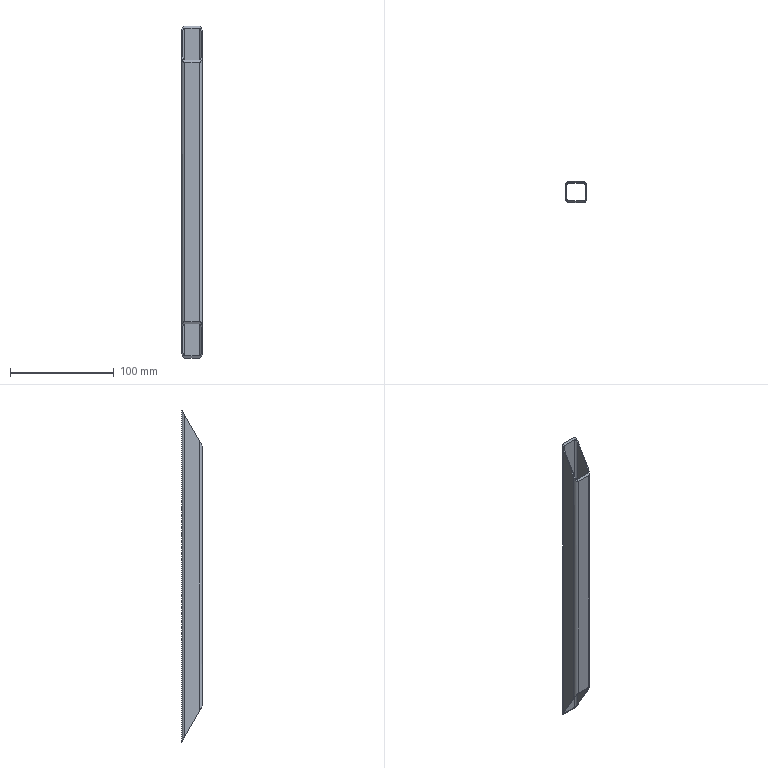Part | SolidWorks | features BaseBody 1 | 1 solid | 18 faces | box 20 x 20 x 320.082 mm | volume 24308 mm3 | plane 10 | cylinder 8 | commonest cylinder face diameters 3.6 x4 6 x4
STEP:
#1=CARTESIAN_POINT('',(7.,10.,0.));
#2=VERTEX_POINT('',#1);
#3=CARTESIAN_POINT('',(-7.,10.,0.));
#4=VERTEX_POINT('',#3);
#5=CARTESIAN_POINT('',(-7.,10.,0.));
#6=DIRECTION('',(-1.,0.,0.));
#7=VECTOR('',#6,1000.);
#8=LINE('',#5,#7);
#9=EDGE_CURVE('',#2,#4,#8,.T.);
#10=ORIENTED_EDGE('',*,*,#9,.T.);
#11=CARTESIAN_POINT('',(-7.,10.,320.082));
#12=VERTEX_POINT('',#11);
#13=CARTESIAN_POINT('',(-7.,10.,0.));
#14=DIRECTION('',(0.,0.,1.));
#15=VECTOR('',#14,1000.);
#16=LINE('',#13,#15);
#17=EDGE_CURVE('',#4,#12,#16,.T.);
#18=ORIENTED_EDGE('',*,*,#17,.T.);
#19=CARTESIAN_POINT('',(7.,10.,320.082));
#20=VERTEX_POINT('',#19);
#21=CARTESIAN_POINT('',(-7.,10.,320.082));
#22=DIRECTION('',(1.,0.,0.));
#23=VECTOR('',#22,1000.);
#24=LINE('',#21,#23);
#25=EDGE_CURVE('',#12,#20,#24,.T.);
#26=ORIENTED_EDGE('',*,*,#25,.T.);
#27=CARTESIAN_POINT('',(7.,10.,0.));
#28=DIRECTION('',(0.,0.,-1.));
#29=VECTOR('',#28,1000.);
#30=LINE('',#27,#29);
#31=EDGE_CURVE('',#20,#2,#30,.T.);
#32=ORIENTED_EDGE('',*,*,#31,.T.);
#33=EDGE_LOOP('',(#10,#18,#26,#32));
#34=FACE_OUTER_BOUND('',#33,.T.);
#35=CARTESIAN_POINT('',(-7.,10.,0.));
#36=DIRECTION('',(0.,1.,0.));
#37=DIRECTION('',(-1.,0.,0.));
#38=AXIS2_PLACEMENT_3D('',#35,#36,#37);
#39=PLANE('',#38);
#40=ADVANCED_FACE('',(#34),#39,.T.);
#41=CARTESIAN_POINT('',(-10.,7.,314.818));
#42=VERTEX_POINT('',#41);
#43=CARTESIAN_POINT('',(-10.,7.,314.818));
#44=CARTESIAN_POINT('',(-10.,8.757,317.902));
#45=CARTESIAN_POINT('',(-8.757,10.,320.082));
#46=CARTESIAN_POINT('',(-7.,10.,320.082));
#47=(BOUNDED_CURVE()B_SPLINE_CURVE(3,(#43,#44,#45,#46),.UNSPECIFIED.,.F.,.F.)B_SPLINE_CURVE_WITH_KNOTS((4,4),(4.712,6.283),.UNSPECIFIED.)CURVE()GEOMETRIC_REPRESENTATION_ITEM()RATIONAL_B_SPLINE_CURVE((1.,0.8047,0.8047,1.))REPRESENTATION_ITEM(''));
#48=EDGE_CURVE('',#42,#12,#47,.T.);
#49=ORIENTED_EDGE('',*,*,#48,.T.);
#50=ORIENTED_EDGE('',*,*,#17,.F.);
#51=CARTESIAN_POINT('',(-10.,7.,5.264));
#52=VERTEX_POINT('',#51);
#53=CARTESIAN_POINT('',(-7.,10.,0.));
#54=CARTESIAN_POINT('',(-8.757,10.,0.));
#55=CARTESIAN_POINT('',(-10.,8.757,2.181));
#56=CARTESIAN_POINT('',(-10.,7.,5.264));
#57=(BOUNDED_CURVE()B_SPLINE_CURVE(3,(#53,#54,#55,#56),.UNSPECIFIED.,.F.,.F.)B_SPLINE_CURVE_WITH_KNOTS((4,4),(3.142,4.712),.UNSPECIFIED.)CURVE()GEOMETRIC_REPRESENTATION_ITEM()RATIONAL_B_SPLINE_CURVE((1.,0.8047,0.8047,1.))REPRESENTATION_ITEM(''));
#58=EDGE_CURVE('',#4,#52,#57,.T.);
#59=ORIENTED_EDGE('',*,*,#58,.T.);
#60=CARTESIAN_POINT('',(-10.,7.,0.));
#61=DIRECTION('',(0.,0.,1.));
#62=VECTOR('',#61,1000.);
#63=LINE('',#60,#62);
#64=EDGE_CURVE('',#52,#42,#63,.T.);
#65=ORIENTED_EDGE('',*,*,#64,.T.);
#66=EDGE_LOOP('',(#49,#50,#59,#65));
#67=FACE_OUTER_BOUND('',#66,.T.);
#68=CARTESIAN_POINT('',(-7.,7.,0.));
#69=DIRECTION('',(0.,0.,1.));
#70=DIRECTION('',(1.,0.,0.));
#71=AXIS2_PLACEMENT_3D('',#68,#69,#70);
#72=CYLINDRICAL_SURFACE('',#71,3.);
#73=ADVANCED_FACE('',(#67),#72,.T.);
#74=CARTESIAN_POINT('',(-8.8,7.,5.264));
#75=VERTEX_POINT('',#74);
#76=CARTESIAN_POINT('',(-7.,8.8,2.106));
#77=VERTEX_POINT('',#76);
#78=CARTESIAN_POINT('',(-8.8,7.,5.264));
#79=CARTESIAN_POINT('',(-8.8,8.054,3.414));
#80=CARTESIAN_POINT('',(-8.054,8.8,2.106));
#81=CARTESIAN_POINT('',(-7.,8.8,2.106));
#82=(BOUNDED_CURVE()B_SPLINE_CURVE(3,(#78,#79,#80,#81),.UNSPECIFIED.,.F.,.F.)B_SPLINE_CURVE_WITH_KNOTS((4,4),(1.571,3.142),.UNSPECIFIED.)CURVE()GEOMETRIC_REPRESENTATION_ITEM()RATIONAL_B_SPLINE_CURVE((1.,0.8047,0.8047,1.))REPRESENTATION_ITEM(''));
#83=EDGE_CURVE('',#75,#77,#82,.T.);
#84=ORIENTED_EDGE('',*,*,#83,.F.);
#85=CARTESIAN_POINT('',(-8.8,-7.,29.831));
#86=VERTEX_POINT('',#85);
#87=CARTESIAN_POINT('',(-8.8,7.549,4.302));
#88=DIRECTION('',(0.,0.4951,-0.8688));
#89=VECTOR('',#88,1000.);
#90=LINE('',#87,#89);
#91=EDGE_CURVE('',#86,#75,#90,.T.);
#92=ORIENTED_EDGE('',*,*,#91,.F.);
#93=CARTESIAN_POINT('',(-7.,-8.8,32.99));
#94=VERTEX_POINT('',#93);
#95=CARTESIAN_POINT('',(-7.,-8.8,32.99));
#96=CARTESIAN_POINT('',(-8.054,-8.8,32.99));
#97=CARTESIAN_POINT('',(-8.8,-8.054,31.682));
#98=CARTESIAN_POINT('',(-8.8,-7.,29.831));
#99=(BOUNDED_CURVE()B_SPLINE_CURVE(3,(#95,#96,#97,#98),.UNSPECIFIED.,.F.,.F.)B_SPLINE_CURVE_WITH_KNOTS((4,4),(0.,1.571),.UNSPECIFIED.)CURVE()GEOMETRIC_REPRESENTATION_ITEM()RATIONAL_B_SPLINE_CURVE((1.,0.8047,0.8047,1.))REPRESENTATION_ITEM(''));
#100=EDGE_CURVE('',#94,#86,#99,.T.);
#101=ORIENTED_EDGE('',*,*,#100,.F.);
#102=CARTESIAN_POINT('',(7.,-8.8,32.99));
#103=VERTEX_POINT('',#102);
#104=CARTESIAN_POINT('',(0.,-8.8,32.99));
#105=DIRECTION('',(-1.,0.,0.));
#106=VECTOR('',#105,1000.);
#107=LINE('',#104,#106);
#108=EDGE_CURVE('',#103,#94,#107,.T.);
#109=ORIENTED_EDGE('',*,*,#108,.F.);
#110=CARTESIAN_POINT('',(8.8,-7.,29.831));
#111=VERTEX_POINT('',#110);
#112=CARTESIAN_POINT('',(8.8,-7.,29.831));
#113=CARTESIAN_POINT('',(8.8,-8.054,31.682));
#114=CARTESIAN_POINT('',(8.054,-8.8,32.99));
#115=CARTESIAN_POINT('',(7.,-8.8,32.99));
#116=(BOUNDED_CURVE()B_SPLINE_CURVE(3,(#112,#113,#114,#115),.UNSPECIFIED.,.F.,.F.)B_SPLINE_CURVE_WITH_KNOTS((4,4),(4.712,6.283),.UNSPECIFIED.)CURVE()GEOMETRIC_REPRESENTATION_ITEM()RATIONAL_B_SPLINE_CURVE((1.,0.8047,0.8047,1.))REPRESENTATION_ITEM(''));
#117=EDGE_CURVE('',#111,#103,#116,.T.);
#118=ORIENTED_EDGE('',*,*,#117,.F.);
#119=CARTESIAN_POINT('',(8.8,7.,5.264));
#120=VERTEX_POINT('',#119);
#121=CARTESIAN_POINT('',(8.8,7.549,4.302));
#122=DIRECTION('',(0.,-0.4951,0.8688));
#123=VECTOR('',#122,1000.);
#124=LINE('',#121,#123);
#125=EDGE_CURVE('',#120,#111,#124,.T.);
#126=ORIENTED_EDGE('',*,*,#125,.F.);
#127=CARTESIAN_POINT('',(7.,8.8,2.106));
#128=VERTEX_POINT('',#127);
#129=CARTESIAN_POINT('',(7.,8.8,2.106));
#130=CARTESIAN_POINT('',(8.054,8.8,2.106));
#131=CARTESIAN_POINT('',(8.8,8.054,3.414));
#132=CARTESIAN_POINT('',(8.8,7.,5.264));
#133=(BOUNDED_CURVE()B_SPLINE_CURVE(3,(#129,#130,#131,#132),.UNSPECIFIED.,.F.,.F.)B_SPLINE_CURVE_WITH_KNOTS((4,4),(3.142,4.712),.UNSPECIFIED.)CURVE()GEOMETRIC_REPRESENTATION_ITEM()RATIONAL_B_SPLINE_CURVE((1.,0.8047,0.8047,1.))REPRESENTATION_ITEM(''));
#134=EDGE_CURVE('',#128,#120,#133,.T.);
#135=ORIENTED_EDGE('',*,*,#134,.F.);
#136=CARTESIAN_POINT('',(0.,8.8,2.106));
#137=DIRECTION('',(1.,0.,0.));
#138=VECTOR('',#137,1000.);
#139=LINE('',#136,#138);
#140=EDGE_CURVE('',#77,#128,#139,.T.);
#141=ORIENTED_EDGE('',*,*,#140,.F.);
#142=EDGE_LOOP('',(#84,#92,#101,#109,#118,#126,#135,#141));
#143=FACE_BOUND('',#142,.T.);
#144=CARTESIAN_POINT('',(10.,-7.,29.831));
#145=VERTEX_POINT('',#144);
#146=CARTESIAN_POINT('',(10.,7.,5.264));
#147=VERTEX_POINT('',#146);
#148=CARTESIAN_POINT('',(10.,7.549,4.302));
#149=DIRECTION('',(0.,0.4951,-0.8688));
#150=VECTOR('',#149,1000.);
#151=LINE('',#148,#150);
#152=EDGE_CURVE('',#145,#147,#151,.T.);
#153=ORIENTED_EDGE('',*,*,#152,.F.);
#154=CARTESIAN_POINT('',(7.,-10.,35.096));
#155=VERTEX_POINT('',#154);
#156=CARTESIAN_POINT('',(7.,-10.,35.096));
#157=CARTESIAN_POINT('',(8.757,-10.,35.096));
#158=CARTESIAN_POINT('',(10.,-8.757,32.915));
#159=CARTESIAN_POINT('',(10.,-7.,29.831));
#160=(BOUNDED_CURVE()B_SPLINE_CURVE(3,(#156,#157,#158,#159),.UNSPECIFIED.,.F.,.F.)B_SPLINE_CURVE_WITH_KNOTS((4,4),(0.,1.571),.UNSPECIFIED.)CURVE()GEOMETRIC_REPRESENTATION_ITEM()RATIONAL_B_SPLINE_CURVE((1.,0.8047,0.8047,1.))REPRESENTATION_ITEM(''));
#161=EDGE_CURVE('',#155,#145,#160,.T.);
#162=ORIENTED_EDGE('',*,*,#161,.F.);
#163=CARTESIAN_POINT('',(-7.,-10.,35.096));
#164=VERTEX_POINT('',#163);
#165=CARTESIAN_POINT('',(0.,-10.,35.096));
#166=DIRECTION('',(1.,0.,0.));
#167=VECTOR('',#166,1000.);
#168=LINE('',#165,#167);
#169=EDGE_CURVE('',#164,#155,#168,.T.);
#170=ORIENTED_EDGE('',*,*,#169,.F.);
#171=CARTESIAN_POINT('',(-10.,-7.,29.831));
#172=VERTEX_POINT('',#171);
#173=CARTESIAN_POINT('',(-10.,-7.,29.831));
#174=CARTESIAN_POINT('',(-10.,-8.757,32.915));
#175=CARTESIAN_POINT('',(-8.757,-10.,35.096));
#176=CARTESIAN_POINT('',(-7.,-10.,35.096));
#177=(BOUNDED_CURVE()B_SPLINE_CURVE(3,(#173,#174,#175,#176),.UNSPECIFIED.,.F.,.T.)B_SPLINE_CURVE_WITH_KNOTS((4,4),(4.712,6.283),.UNSPECIFIED.)CURVE()GEOMETRIC_REPRESENTATION_ITEM()RATIONAL_B_SPLINE_CURVE((1.,0.8047,0.8047,1.))REPRESENTATION_ITEM(''));
#178=EDGE_CURVE('',#172,#164,#177,.T.);
#179=ORIENTED_EDGE('',*,*,#178,.F.);
#180=CARTESIAN_POINT('',(-10.,7.549,4.302));
#181=DIRECTION('',(0.,-0.4951,0.8688));
#182=VECTOR('',#181,1000.);
#183=LINE('',#180,#182);
#184=EDGE_CURVE('',#52,#172,#183,.T.);
#185=ORIENTED_EDGE('',*,*,#184,.F.);
#186=ORIENTED_EDGE('',*,*,#58,.F.);
#187=ORIENTED_EDGE('',*,*,#9,.F.);
#188=CARTESIAN_POINT('',(10.,7.,5.264));
#189=CARTESIAN_POINT('',(10.,8.757,2.181));
#190=CARTESIAN_POINT('',(8.757,10.,0.));
#191=CARTESIAN_POINT('',(7.,10.,0.));
#192=(BOUNDED_CURVE()B_SPLINE_CURVE(3,(#188,#189,#190,#191),.UNSPECIFIED.,.F.,.F.)B_SPLINE_CURVE_WITH_KNOTS((4,4),(1.571,3.142),.UNSPECIFIED.)CURVE()GEOMETRIC_REPRESENTATION_ITEM()RATIONAL_B_SPLINE_CURVE((1.,0.8047,0.8047,1.))REPRESENTATION_ITEM(''));
#193=EDGE_CURVE('',#147,#2,#192,.T.);
#194=ORIENTED_EDGE('',*,*,#193,.F.);
#195=EDGE_LOOP('',(#153,#162,#170,#179,#185,#186,#187,#194));
#196=FACE_OUTER_BOUND('',#195,.T.);
#197=CARTESIAN_POINT('',(0.,7.549,4.302));
#198=DIRECTION('',(0.,0.8688,0.4951));
#199=DIRECTION('',(0.,-0.4951,0.8688));
#200=AXIS2_PLACEMENT_3D('',#197,#198,#199);
#201=PLANE('',#200);
#202=ADVANCED_FACE('',(#143,#196),#201,.F.);
#203=CARTESIAN_POINT('',(10.,7.,314.818));
#204=VERTEX_POINT('',#203);
#205=CARTESIAN_POINT('',(7.,10.,320.082));
#206=CARTESIAN_POINT('',(8.757,10.,320.082));
#207=CARTESIAN_POINT('',(10.,8.757,317.902));
#208=CARTESIAN_POINT('',(10.,7.,314.818));
#209=(BOUNDED_CURVE()B_SPLINE_CURVE(3,(#205,#206,#207,#208),.UNSPECIFIED.,.F.,.F.)B_SPLINE_CURVE_WITH_KNOTS((4,4),(0.,1.571),.UNSPECIFIED.)CURVE()GEOMETRIC_REPRESENTATION_ITEM()RATIONAL_B_SPLINE_CURVE((1.,0.8047,0.8047,1.))REPRESENTATION_ITEM(''));
#210=EDGE_CURVE('',#20,#204,#209,.T.);
#211=ORIENTED_EDGE('',*,*,#210,.T.);
#212=CARTESIAN_POINT('',(10.,7.,0.));
#213=DIRECTION('',(0.,0.,-1.));
#214=VECTOR('',#213,1000.);
#215=LINE('',#212,#214);
#216=EDGE_CURVE('',#204,#147,#215,.T.);
#217=ORIENTED_EDGE('',*,*,#216,.T.);
#218=ORIENTED_EDGE('',*,*,#193,.T.);
#219=ORIENTED_EDGE('',*,*,#31,.F.);
#220=EDGE_LOOP('',(#211,#217,#218,#219));
#221=FACE_OUTER_BOUND('',#220,.T.);
#222=CARTESIAN_POINT('',(7.,7.,0.));
#223=DIRECTION('',(0.,0.,1.));
#224=DIRECTION('',(1.,0.,0.));
#225=AXIS2_PLACEMENT_3D('',#222,#223,#224);
#226=CYLINDRICAL_SURFACE('',#225,3.);
#227=ADVANCED_FACE('',(#221),#226,.T.);
#228=CARTESIAN_POINT('',(-8.8,-7.,290.257));
#229=VERTEX_POINT('',#228);
#230=CARTESIAN_POINT('',(-7.,-8.8,287.099));
#231=VERTEX_POINT('',#230);
#232=CARTESIAN_POINT('',(-8.8,-7.,290.257));
#233=CARTESIAN_POINT('',(-8.8,-8.054,288.407));
#234=CARTESIAN_POINT('',(-8.054,-8.8,287.099));
#235=CARTESIAN_POINT('',(-7.,-8.8,287.099));
#236=(BOUNDED_CURVE()B_SPLINE_CURVE(3,(#232,#233,#234,#235),.UNSPECIFIED.,.F.,.F.)B_SPLINE_CURVE_WITH_KNOTS((4,4),(1.571,3.142),.UNSPECIFIED.)CURVE()GEOMETRIC_REPRESENTATION_ITEM()RATIONAL_B_SPLINE_CURVE((1.,0.8047,0.8047,1.))REPRESENTATION_ITEM(''));
#237=EDGE_CURVE('',#229,#231,#236,.T.);
#238=ORIENTED_EDGE('',*,*,#237,.F.);
#239=CARTESIAN_POINT('',(-8.8,7.,314.818));
#240=VERTEX_POINT('',#239);
#241=CARTESIAN_POINT('',(-8.8,-130.158,74.19));
#242=DIRECTION('',(0.,-0.4952,-0.8688));
#243=VECTOR('',#242,1000.);
#244=LINE('',#241,#243);
#245=EDGE_CURVE('',#240,#229,#244,.T.);
#246=ORIENTED_EDGE('',*,*,#245,.F.);
#247=CARTESIAN_POINT('',(-7.,8.8,317.976));
#248=VERTEX_POINT('',#247);
#249=CARTESIAN_POINT('',(-7.,8.8,317.976));
#250=CARTESIAN_POINT('',(-8.054,8.8,317.976));
#251=CARTESIAN_POINT('',(-8.8,8.054,316.668));
#252=CARTESIAN_POINT('',(-8.8,7.,314.818));
#253=(BOUNDED_CURVE()B_SPLINE_CURVE(3,(#249,#250,#251,#252),.UNSPECIFIED.,.F.,.F.)B_SPLINE_CURVE_WITH_KNOTS((4,4),(0.,1.571),.UNSPECIFIED.)CURVE()GEOMETRIC_REPRESENTATION_ITEM()RATIONAL_B_SPLINE_CURVE((1.,0.8047,0.8047,1.))REPRESENTATION_ITEM(''));
#254=EDGE_CURVE('',#248,#240,#253,.T.);
#255=ORIENTED_EDGE('',*,*,#254,.F.);
#256=CARTESIAN_POINT('',(7.,8.8,317.976));
#257=VERTEX_POINT('',#256);
#258=CARTESIAN_POINT('',(0.,8.8,317.976));
#259=DIRECTION('',(-1.,0.,0.));
#260=VECTOR('',#259,1000.);
#261=LINE('',#258,#260);
#262=EDGE_CURVE('',#257,#248,#261,.T.);
#263=ORIENTED_EDGE('',*,*,#262,.F.);
#264=CARTESIAN_POINT('',(8.8,7.,314.818));
#265=VERTEX_POINT('',#264);
#266=CARTESIAN_POINT('',(8.8,7.,314.818));
#267=CARTESIAN_POINT('',(8.8,8.054,316.668));
#268=CARTESIAN_POINT('',(8.054,8.8,317.976));
#269=CARTESIAN_POINT('',(7.,8.8,317.976));
#270=(BOUNDED_CURVE()B_SPLINE_CURVE(3,(#266,#267,#268,#269),.UNSPECIFIED.,.F.,.F.)B_SPLINE_CURVE_WITH_KNOTS((4,4),(4.712,6.283),.UNSPECIFIED.)CURVE()GEOMETRIC_REPRESENTATION_ITEM()RATIONAL_B_SPLINE_CURVE((1.,0.8047,0.8047,1.))REPRESENTATION_ITEM(''));
#271=EDGE_CURVE('',#265,#257,#270,.T.);
#272=ORIENTED_EDGE('',*,*,#271,.F.);
#273=CARTESIAN_POINT('',(8.8,-7.,290.257));
#274=VERTEX_POINT('',#273);
#275=CARTESIAN_POINT('',(8.8,-130.158,74.19));
#276=DIRECTION('',(0.,0.4952,0.8688));
#277=VECTOR('',#276,1000.);
#278=LINE('',#275,#277);
#279=EDGE_CURVE('',#274,#265,#278,.T.);
#280=ORIENTED_EDGE('',*,*,#279,.F.);
#281=CARTESIAN_POINT('',(7.,-8.8,287.099));
#282=VERTEX_POINT('',#281);
#283=CARTESIAN_POINT('',(7.,-8.8,287.099));
#284=CARTESIAN_POINT('',(8.054,-8.8,287.099));
#285=CARTESIAN_POINT('',(8.8,-8.054,288.407));
#286=CARTESIAN_POINT('',(8.8,-7.,290.257));
#287=(BOUNDED_CURVE()B_SPLINE_CURVE(3,(#283,#284,#285,#286),.UNSPECIFIED.,.F.,.T.)B_SPLINE_CURVE_WITH_KNOTS((4,4),(3.142,4.712),.UNSPECIFIED.)CURVE()GEOMETRIC_REPRESENTATION_ITEM()RATIONAL_B_SPLINE_CURVE((1.,0.8047,0.8047,1.))REPRESENTATION_ITEM(''));
#288=EDGE_CURVE('',#282,#274,#287,.T.);
#289=ORIENTED_EDGE('',*,*,#288,.F.);
#290=CARTESIAN_POINT('',(0.,-8.8,287.099));
#291=DIRECTION('',(1.,0.,0.));
#292=VECTOR('',#291,1000.);
#293=LINE('',#290,#292);
#294=EDGE_CURVE('',#231,#282,#293,.T.);
#295=ORIENTED_EDGE('',*,*,#294,.F.);
#296=EDGE_LOOP('',(#238,#246,#255,#263,#272,#280,#289,#295));
#297=FACE_BOUND('',#296,.T.);
#298=ORIENTED_EDGE('',*,*,#210,.F.);
#299=ORIENTED_EDGE('',*,*,#25,.F.);
#300=ORIENTED_EDGE('',*,*,#48,.F.);
#301=CARTESIAN_POINT('',(-10.,-7.,290.257));
#302=VERTEX_POINT('',#301);
#303=CARTESIAN_POINT('',(-10.,-130.158,74.19));
#304=DIRECTION('',(0.,0.4952,0.8688));
#305=VECTOR('',#304,1000.);
#306=LINE('',#303,#305);
#307=EDGE_CURVE('',#302,#42,#306,.T.);
#308=ORIENTED_EDGE('',*,*,#307,.F.);
#309=CARTESIAN_POINT('',(-7.,-10.,284.994));
#310=VERTEX_POINT('',#309);
#311=CARTESIAN_POINT('',(-7.,-10.,284.994));
#312=CARTESIAN_POINT('',(-8.757,-10.,284.994));
#313=CARTESIAN_POINT('',(-10.,-8.757,287.174));
#314=CARTESIAN_POINT('',(-10.,-7.,290.257));
#315=(BOUNDED_CURVE()B_SPLINE_CURVE(3,(#311,#312,#313,#314),.UNSPECIFIED.,.F.,.F.)B_SPLINE_CURVE_WITH_KNOTS((4,4),(3.142,4.712),.UNSPECIFIED.)CURVE()GEOMETRIC_REPRESENTATION_ITEM()RATIONAL_B_SPLINE_CURVE((1.,0.8047,0.8047,1.))REPRESENTATION_ITEM(''));
#316=EDGE_CURVE('',#310,#302,#315,.T.);
#317=ORIENTED_EDGE('',*,*,#316,.F.);
#318=CARTESIAN_POINT('',(7.,-10.,284.994));
#319=VERTEX_POINT('',#318);
#320=CARTESIAN_POINT('',(0.,-10.,284.994));
#321=DIRECTION('',(-1.,0.,0.));
#322=VECTOR('',#321,1000.);
#323=LINE('',#320,#322);
#324=EDGE_CURVE('',#319,#310,#323,.T.);
#325=ORIENTED_EDGE('',*,*,#324,.F.);
#326=CARTESIAN_POINT('',(10.,-7.,290.257));
#327=VERTEX_POINT('',#326);
#328=CARTESIAN_POINT('',(10.,-7.,290.257));
#329=CARTESIAN_POINT('',(10.,-8.757,287.174));
#330=CARTESIAN_POINT('',(8.757,-10.,284.994));
#331=CARTESIAN_POINT('',(7.,-10.,284.994));
#332=(BOUNDED_CURVE()B_SPLINE_CURVE(3,(#328,#329,#330,#331),.UNSPECIFIED.,.F.,.F.)B_SPLINE_CURVE_WITH_KNOTS((4,4),(1.571,3.142),.UNSPECIFIED.)CURVE()GEOMETRIC_REPRESENTATION_ITEM()RATIONAL_B_SPLINE_CURVE((1.,0.8047,0.8047,1.))REPRESENTATION_ITEM(''));
#333=EDGE_CURVE('',#327,#319,#332,.T.);
#334=ORIENTED_EDGE('',*,*,#333,.F.);
#335=CARTESIAN_POINT('',(10.,-130.158,74.19));
#336=DIRECTION('',(0.,-0.4952,-0.8688));
#337=VECTOR('',#336,1000.);
#338=LINE('',#335,#337);
#339=EDGE_CURVE('',#204,#327,#338,.T.);
#340=ORIENTED_EDGE('',*,*,#339,.F.);
#341=EDGE_LOOP('',(#298,#299,#300,#308,#317,#325,#334,#340));
#342=FACE_OUTER_BOUND('',#341,.T.);
#343=CARTESIAN_POINT('',(0.,-130.158,74.19));
#344=DIRECTION('',(0.,0.8688,-0.4952));
#345=DIRECTION('',(0.,0.4952,0.8688));
#346=AXIS2_PLACEMENT_3D('',#343,#344,#345);
#347=PLANE('',#346);
#348=ADVANCED_FACE('',(#297,#342),#347,.F.);
#349=ORIENTED_EDGE('',*,*,#307,.T.);
#350=ORIENTED_EDGE('',*,*,#64,.F.);
#351=ORIENTED_EDGE('',*,*,#184,.T.);
#352=CARTESIAN_POINT('',(-10.,-7.,0.));
#353=DIRECTION('',(0.,0.,1.));
#354=VECTOR('',#353,1000.);
#355=LINE('',#352,#354);
#356=EDGE_CURVE('',#172,#302,#355,.T.);
#357=ORIENTED_EDGE('',*,*,#356,.T.);
#358=EDGE_LOOP('',(#349,#350,#351,#357));
#359=FACE_OUTER_BOUND('',#358,.T.);
#360=CARTESIAN_POINT('',(-10.,-7.,0.));
#361=DIRECTION('',(-1.,0.,0.));
#362=DIRECTION('',(0.,-1.,0.));
#363=AXIS2_PLACEMENT_3D('',#360,#361,#362);
#364=PLANE('',#363);
#365=ADVANCED_FACE('',(#359),#364,.T.);
#366=CARTESIAN_POINT('',(7.,8.8,0.));
#367=DIRECTION('',(0.,0.,-1.));
#368=VECTOR('',#367,1000.);
#369=LINE('',#366,#368);
#370=EDGE_CURVE('',#257,#128,#369,.T.);
#371=ORIENTED_EDGE('',*,*,#370,.F.);
#372=ORIENTED_EDGE('',*,*,#262,.T.);
#373=CARTESIAN_POINT('',(-7.,8.8,0.));
#374=DIRECTION('',(0.,0.,1.));
#375=VECTOR('',#374,1000.);
#376=LINE('',#373,#375);
#377=EDGE_CURVE('',#77,#248,#376,.T.);
#378=ORIENTED_EDGE('',*,*,#377,.F.);
#379=ORIENTED_EDGE('',*,*,#140,.T.);
#380=EDGE_LOOP('',(#371,#372,#378,#379));
#381=FACE_OUTER_BOUND('',#380,.T.);
#382=CARTESIAN_POINT('',(-7.,8.8,0.));
#383=DIRECTION('',(0.,1.,0.));
#384=DIRECTION('',(-1.,0.,0.));
#385=AXIS2_PLACEMENT_3D('',#382,#383,#384);
#386=PLANE('',#385);
#387=ADVANCED_FACE('',(#381),#386,.F.);
#388=ORIENTED_EDGE('',*,*,#377,.T.);
#389=ORIENTED_EDGE('',*,*,#254,.T.);
#390=CARTESIAN_POINT('',(-8.8,7.,0.));
#391=DIRECTION('',(0.,0.,1.));
#392=VECTOR('',#391,1000.);
#393=LINE('',#390,#392);
#394=EDGE_CURVE('',#75,#240,#393,.T.);
#395=ORIENTED_EDGE('',*,*,#394,.F.);
#396=ORIENTED_EDGE('',*,*,#83,.T.);
#397=EDGE_LOOP('',(#388,#389,#395,#396));
#398=FACE_OUTER_BOUND('',#397,.T.);
#399=CARTESIAN_POINT('',(-7.,7.,0.));
#400=DIRECTION('',(0.,0.,1.));
#401=DIRECTION('',(1.,0.,0.));
#402=AXIS2_PLACEMENT_3D('',#399,#400,#401);
#403=CYLINDRICAL_SURFACE('',#402,1.8);
#404=ADVANCED_FACE('',(#398),#403,.F.);
#405=ORIENTED_EDGE('',*,*,#394,.T.);
#406=ORIENTED_EDGE('',*,*,#245,.T.);
#407=CARTESIAN_POINT('',(-8.8,-7.,0.));
#408=DIRECTION('',(0.,0.,1.));
#409=VECTOR('',#408,1000.);
#410=LINE('',#407,#409);
#411=EDGE_CURVE('',#86,#229,#410,.T.);
#412=ORIENTED_EDGE('',*,*,#411,.F.);
#413=ORIENTED_EDGE('',*,*,#91,.T.);
#414=EDGE_LOOP('',(#405,#406,#412,#413));
#415=FACE_OUTER_BOUND('',#414,.T.);
#416=CARTESIAN_POINT('',(-8.8,-7.,0.));
#417=DIRECTION('',(-1.,0.,0.));
#418=DIRECTION('',(0.,-1.,0.));
#419=AXIS2_PLACEMENT_3D('',#416,#417,#418);
#420=PLANE('',#419);
#421=ADVANCED_FACE('',(#415),#420,.F.);
#422=ORIENTED_EDGE('',*,*,#411,.T.);
#423=ORIENTED_EDGE('',*,*,#237,.T.);
#424=CARTESIAN_POINT('',(-7.,-8.8,0.));
#425=DIRECTION('',(0.,0.,1.));
#426=VECTOR('',#425,1000.);
#427=LINE('',#424,#426);
#428=EDGE_CURVE('',#94,#231,#427,.T.);
#429=ORIENTED_EDGE('',*,*,#428,.F.);
#430=ORIENTED_EDGE('',*,*,#100,.T.);
#431=EDGE_LOOP('',(#422,#423,#429,#430));
#432=FACE_OUTER_BOUND('',#431,.T.);
#433=CARTESIAN_POINT('',(-7.,-7.,0.));
#434=DIRECTION('',(0.,0.,1.));
#435=DIRECTION('',(1.,0.,0.));
#436=AXIS2_PLACEMENT_3D('',#433,#434,#435);
#437=CYLINDRICAL_SURFACE('',#436,1.8);
#438=ADVANCED_FACE('',(#432),#437,.F.);
#439=ORIENTED_EDGE('',*,*,#428,.T.);
#440=ORIENTED_EDGE('',*,*,#294,.T.);
#441=CARTESIAN_POINT('',(7.,-8.8,0.));
#442=DIRECTION('',(0.,0.,1.));
#443=VECTOR('',#442,1000.);
#444=LINE('',#441,#443);
#445=EDGE_CURVE('',#103,#282,#444,.T.);
#446=ORIENTED_EDGE('',*,*,#445,.F.);
#447=ORIENTED_EDGE('',*,*,#108,.T.);
#448=EDGE_LOOP('',(#439,#440,#446,#447));
#449=FACE_OUTER_BOUND('',#448,.T.);
#450=CARTESIAN_POINT('',(7.,-8.8,0.));
#451=DIRECTION('',(0.,-1.,0.));
#452=DIRECTION('',(1.,0.,0.));
#453=AXIS2_PLACEMENT_3D('',#450,#451,#452);
#454=PLANE('',#453);
#455=ADVANCED_FACE('',(#449),#454,.F.);
#456=ORIENTED_EDGE('',*,*,#445,.T.);
#457=ORIENTED_EDGE('',*,*,#288,.T.);
#458=CARTESIAN_POINT('',(8.8,-7.,0.));
#459=DIRECTION('',(0.,0.,1.));
#460=VECTOR('',#459,1000.);
#461=LINE('',#458,#460);
#462=EDGE_CURVE('',#111,#274,#461,.T.);
#463=ORIENTED_EDGE('',*,*,#462,.F.);
#464=ORIENTED_EDGE('',*,*,#117,.T.);
#465=EDGE_LOOP('',(#456,#457,#463,#464));
#466=FACE_OUTER_BOUND('',#465,.T.);
#467=CARTESIAN_POINT('',(7.,-7.,0.));
#468=DIRECTION('',(0.,0.,1.));
#469=DIRECTION('',(1.,0.,0.));
#470=AXIS2_PLACEMENT_3D('',#467,#468,#469);
#471=CYLINDRICAL_SURFACE('',#470,1.8);
#472=ADVANCED_FACE('',(#466),#471,.F.);
#473=ORIENTED_EDGE('',*,*,#462,.T.);
#474=ORIENTED_EDGE('',*,*,#279,.T.);
#475=CARTESIAN_POINT('',(8.8,7.,0.));
#476=DIRECTION('',(0.,0.,1.));
#477=VECTOR('',#476,1000.);
#478=LINE('',#475,#477);
#479=EDGE_CURVE('',#120,#265,#478,.T.);
#480=ORIENTED_EDGE('',*,*,#479,.F.);
#481=ORIENTED_EDGE('',*,*,#125,.T.);
#482=EDGE_LOOP('',(#473,#474,#480,#481));
#483=FACE_OUTER_BOUND('',#482,.T.);
#484=CARTESIAN_POINT('',(8.8,7.,0.));
#485=DIRECTION('',(1.,0.,0.));
#486=DIRECTION('',(0.,0.,-1.));
#487=AXIS2_PLACEMENT_3D('',#484,#485,#486);
#488=PLANE('',#487);
#489=ADVANCED_FACE('',(#483),#488,.F.);
#490=ORIENTED_EDGE('',*,*,#479,.T.);
#491=ORIENTED_EDGE('',*,*,#271,.T.);
#492=ORIENTED_EDGE('',*,*,#370,.T.);
#493=ORIENTED_EDGE('',*,*,#134,.T.);
#494=EDGE_LOOP('',(#490,#491,#492,#493));
#495=FACE_OUTER_BOUND('',#494,.T.);
#496=CARTESIAN_POINT('',(7.,7.,0.));
#497=DIRECTION('',(0.,0.,1.));
#498=DIRECTION('',(1.,0.,0.));
#499=AXIS2_PLACEMENT_3D('',#496,#497,#498);
#500=CYLINDRICAL_SURFACE('',#499,1.8);
#501=ADVANCED_FACE('',(#495),#500,.F.);
#502=ORIENTED_EDGE('',*,*,#339,.T.);
#503=CARTESIAN_POINT('',(10.,-7.,0.));
#504=DIRECTION('',(0.,0.,-1.));
#505=VECTOR('',#504,1000.);
#506=LINE('',#503,#505);
#507=EDGE_CURVE('',#327,#145,#506,.T.);
#508=ORIENTED_EDGE('',*,*,#507,.T.);
#509=ORIENTED_EDGE('',*,*,#152,.T.);
#510=ORIENTED_EDGE('',*,*,#216,.F.);
#511=EDGE_LOOP('',(#502,#508,#509,#510));
#512=FACE_OUTER_BOUND('',#511,.T.);
#513=CARTESIAN_POINT('',(10.,7.,0.));
#514=DIRECTION('',(1.,0.,0.));
#515=DIRECTION('',(0.,0.,-1.));
#516=AXIS2_PLACEMENT_3D('',#513,#514,#515);
#517=PLANE('',#516);
#518=ADVANCED_FACE('',(#512),#517,.T.);
#519=ORIENTED_EDGE('',*,*,#333,.T.);
#520=CARTESIAN_POINT('',(7.,-10.,0.));
#521=DIRECTION('',(0.,0.,-1.));
#522=VECTOR('',#521,1000.);
#523=LINE('',#520,#522);
#524=EDGE_CURVE('',#319,#155,#523,.T.);
#525=ORIENTED_EDGE('',*,*,#524,.T.);
#526=ORIENTED_EDGE('',*,*,#161,.T.);
#527=ORIENTED_EDGE('',*,*,#507,.F.);
#528=EDGE_LOOP('',(#519,#525,#526,#527));
#529=FACE_OUTER_BOUND('',#528,.T.);
#530=CARTESIAN_POINT('',(7.,-7.,0.));
#531=DIRECTION('',(0.,0.,1.));
#532=DIRECTION('',(1.,0.,0.));
#533=AXIS2_PLACEMENT_3D('',#530,#531,#532);
#534=CYLINDRICAL_SURFACE('',#533,3.);
#535=ADVANCED_FACE('',(#529),#534,.T.);
#536=ORIENTED_EDGE('',*,*,#324,.T.);
#537=CARTESIAN_POINT('',(-7.,-10.,0.));
#538=DIRECTION('',(0.,0.,-1.));
#539=VECTOR('',#538,1000.);
#540=LINE('',#537,#539);
#541=EDGE_CURVE('',#310,#164,#540,.T.);
#542=ORIENTED_EDGE('',*,*,#541,.T.);
#543=ORIENTED_EDGE('',*,*,#169,.T.);
#544=ORIENTED_EDGE('',*,*,#524,.F.);
#545=EDGE_LOOP('',(#536,#542,#543,#544));
#546=FACE_OUTER_BOUND('',#545,.T.);
#547=CARTESIAN_POINT('',(7.,-10.,0.));
#548=DIRECTION('',(0.,-1.,0.));
#549=DIRECTION('',(1.,0.,0.));
#550=AXIS2_PLACEMENT_3D('',#547,#548,#549);
#551=PLANE('',#550);
#552=ADVANCED_FACE('',(#546),#551,.T.);
#553=ORIENTED_EDGE('',*,*,#316,.T.);
#554=ORIENTED_EDGE('',*,*,#356,.F.);
#555=ORIENTED_EDGE('',*,*,#178,.T.);
#556=ORIENTED_EDGE('',*,*,#541,.F.);
#557=EDGE_LOOP('',(#553,#554,#555,#556));
#558=FACE_OUTER_BOUND('',#557,.T.);
#559=CARTESIAN_POINT('',(-7.,-7.,0.));
#560=DIRECTION('',(0.,0.,1.));
#561=DIRECTION('',(1.,0.,0.));
#562=AXIS2_PLACEMENT_3D('',#559,#560,#561);
#563=CYLINDRICAL_SURFACE('',#562,3.);
#564=ADVANCED_FACE('',(#558),#563,.T.);
#565=CLOSED_SHELL('',(#40,#73,#202,#227,#348,#365,#387,#404,#421,#438,#455,#472,#489,#501,#518,#535,#552,#564));
#566=MANIFOLD_SOLID_BREP('',#565);
#567=CARTESIAN_POINT('',(0.,0.,0.));
#568=DIRECTION('',(0.,0.,1.));
#569=DIRECTION('',(1.,0.,0.));
#570=AXIS2_PLACEMENT_3D('',#567,#568,#569);
#571=(LENGTH_UNIT()NAMED_UNIT(*)SI_UNIT(.MILLI.,.METRE.));
#572=UNCERTAINTY_MEASURE_WITH_UNIT(LENGTH_MEASURE(0.00001),#571,'','');
#573=(NAMED_UNIT(*)PLANE_ANGLE_UNIT()SI_UNIT($,.RADIAN.));
#574=(NAMED_UNIT(*)SI_UNIT($,.STERADIAN.)SOLID_ANGLE_UNIT());
#575=(GEOMETRIC_REPRESENTATION_CONTEXT(3)GLOBAL_UNCERTAINTY_ASSIGNED_CONTEXT((#572))GLOBAL_UNIT_ASSIGNED_CONTEXT((#571,#573,#574))REPRESENTATION_CONTEXT('',''));
#576=ADVANCED_BREP_SHAPE_REPRESENTATION('',(#566,#570),#575);